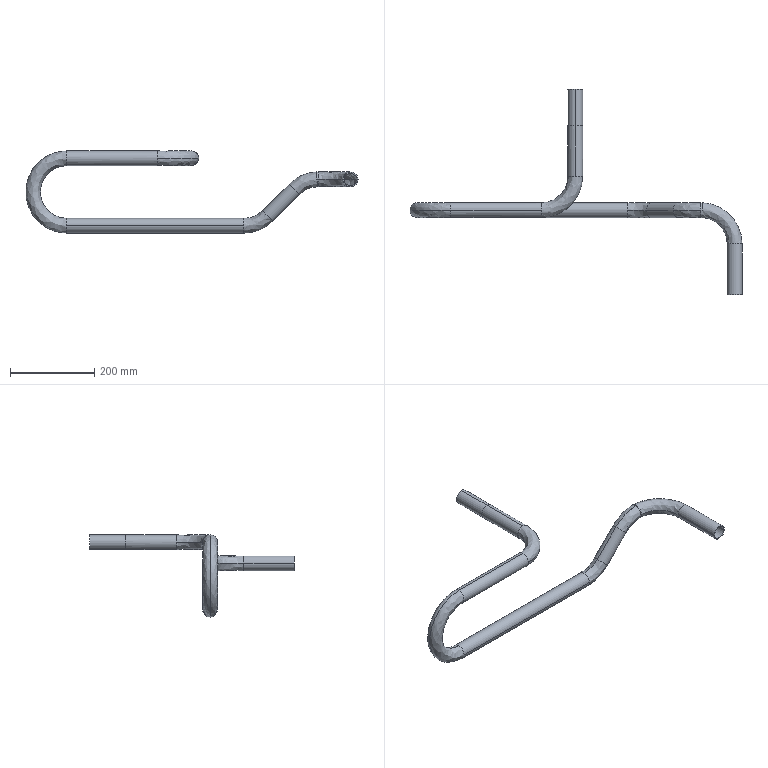Part | STEP file | copper tube 22_default_machined_ | 2 solids | 52 faces | box 787.8 x 486 x 195 mm | volume 412220 mm3 | cylinder 24 | spline 20 | plane 8 | commonest cylinder face diameters 35 x14 31 x10